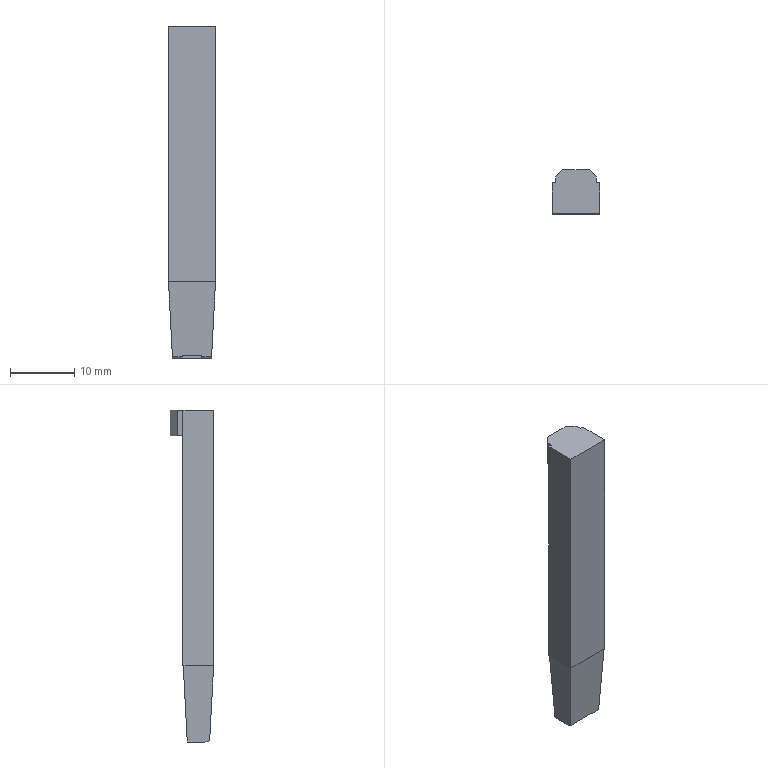Part | Creo | 1 solid | 23 faces | box 7.421 x 6.821 x 51.658 mm | volume 1794 mm3 | plane 23
STEP:
#1=CARTESIAN_POINT('',(0.,0.,0.));
#2=DIRECTION('',(0.,0.,1.));
#3=DIRECTION('',(1.,0.,0.));
#4=AXIS2_PLACEMENT_3D('',#1,#2,#3);
#5=CARTESIAN_POINT('',(22.844,-82.165,46.111));
#6=VERTEX_POINT('',#5);
#7=CARTESIAN_POINT('',(22.844,-86.985,46.111));
#8=VERTEX_POINT('',#7);
#9=CARTESIAN_POINT('',(22.844,-82.165,46.111));
#10=DIRECTION('',(0.,-1.,0.));
#11=VECTOR('',#10,4.821);
#12=LINE('',#9,#11);
#13=EDGE_CURVE('',#6,#8,#12,.T.);
#14=ORIENTED_EDGE('',*,*,#13,.T.);
#15=CARTESIAN_POINT('',(30.265,-86.985,46.111));
#16=VERTEX_POINT('',#15);
#17=CARTESIAN_POINT('',(30.265,-86.985,46.111));
#18=DIRECTION('',(-1.,0.,0.));
#19=VECTOR('',#18,7.421);
#20=LINE('',#17,#19);
#21=EDGE_CURVE('',#16,#8,#20,.T.);
#22=ORIENTED_EDGE('',*,*,#21,.F.);
#23=CARTESIAN_POINT('',(30.265,-82.165,46.111));
#24=VERTEX_POINT('',#23);
#25=CARTESIAN_POINT('',(30.265,-86.985,46.111));
#26=DIRECTION('',(0.,1.,0.));
#27=VECTOR('',#26,4.821);
#28=LINE('',#25,#27);
#29=EDGE_CURVE('',#16,#24,#28,.T.);
#30=ORIENTED_EDGE('',*,*,#29,.T.);
#31=CARTESIAN_POINT('',(30.265,-82.165,46.111));
#32=DIRECTION('',(-1.,0.,0.));
#33=VECTOR('',#32,7.421);
#34=LINE('',#31,#33);
#35=EDGE_CURVE('',#24,#6,#34,.T.);
#36=ORIENTED_EDGE('',*,*,#35,.T.);
#37=EDGE_LOOP('',(#14,#22,#30,#36));
#38=FACE_OUTER_BOUND('',#37,.F.);
#39=CARTESIAN_POINT('',(30.215,-82.215,46.111));
#40=VERTEX_POINT('',#39);
#41=CARTESIAN_POINT('',(22.894,-82.215,46.111));
#42=VERTEX_POINT('',#41);
#43=CARTESIAN_POINT('',(30.215,-82.215,46.111));
#44=DIRECTION('',(-1.,0.,0.));
#45=VECTOR('',#44,7.321);
#46=LINE('',#43,#45);
#47=EDGE_CURVE('',#40,#42,#46,.T.);
#48=ORIENTED_EDGE('',*,*,#47,.F.);
#49=CARTESIAN_POINT('',(30.215,-86.935,46.111));
#50=VERTEX_POINT('',#49);
#51=CARTESIAN_POINT('',(30.215,-86.935,46.111));
#52=DIRECTION('',(0.,1.,0.));
#53=VECTOR('',#52,4.721);
#54=LINE('',#51,#53);
#55=EDGE_CURVE('',#50,#40,#54,.T.);
#56=ORIENTED_EDGE('',*,*,#55,.F.);
#57=CARTESIAN_POINT('',(22.894,-86.935,46.111));
#58=VERTEX_POINT('',#57);
#59=CARTESIAN_POINT('',(22.894,-86.935,46.111));
#60=DIRECTION('',(1.,0.,0.));
#61=VECTOR('',#60,7.321);
#62=LINE('',#59,#61);
#63=EDGE_CURVE('',#58,#50,#62,.T.);
#64=ORIENTED_EDGE('',*,*,#63,.F.);
#65=CARTESIAN_POINT('',(22.894,-82.215,46.111));
#66=DIRECTION('',(0.,-1.,0.));
#67=VECTOR('',#66,4.721);
#68=LINE('',#65,#67);
#69=EDGE_CURVE('',#42,#58,#68,.T.);
#70=ORIENTED_EDGE('',*,*,#69,.F.);
#71=EDGE_LOOP('',(#48,#56,#64,#70));
#72=FACE_BOUND('',#71,.F.);
#73=CARTESIAN_POINT('',(26.554,-82.215,46.111));
#74=DIRECTION('',(0.,0.,1.));
#75=DIRECTION('',(1.,0.,0.));
#76=AXIS2_PLACEMENT_3D('',#73,#74,#75);
#77=PLANE('',#76);
#78=ADVANCED_FACE('',(#38,#72),#77,.F.);
#79=ORIENTED_EDGE('',*,*,#13,.F.);
#80=CARTESIAN_POINT('',(22.844,-82.165,85.91));
#81=VERTEX_POINT('',#80);
#82=CARTESIAN_POINT('',(22.844,-82.165,85.91));
#83=DIRECTION('',(0.,0.,-1.));
#84=VECTOR('',#83,39.799);
#85=LINE('',#82,#84);
#86=EDGE_CURVE('',#81,#6,#85,.T.);
#87=ORIENTED_EDGE('',*,*,#86,.F.);
#88=CARTESIAN_POINT('',(22.844,-86.985,85.91));
#89=VERTEX_POINT('',#88);
#90=CARTESIAN_POINT('',(22.844,-82.165,85.91));
#91=DIRECTION('',(0.,-1.,0.));
#92=VECTOR('',#91,4.821);
#93=LINE('',#90,#92);
#94=EDGE_CURVE('',#81,#89,#93,.T.);
#95=ORIENTED_EDGE('',*,*,#94,.T.);
#96=CARTESIAN_POINT('',(22.844,-86.985,85.91));
#97=DIRECTION('',(0.,0.,-1.));
#98=VECTOR('',#97,39.799);
#99=LINE('',#96,#98);
#100=EDGE_CURVE('',#89,#8,#99,.T.);
#101=ORIENTED_EDGE('',*,*,#100,.T.);
#102=EDGE_LOOP('',(#79,#87,#95,#101));
#103=FACE_OUTER_BOUND('',#102,.F.);
#104=CARTESIAN_POINT('',(22.844,-84.575,30.111));
#105=DIRECTION('',(-1.,0.,0.));
#106=DIRECTION('',(0.,0.,1.));
#107=AXIS2_PLACEMENT_3D('',#104,#105,#106);
#108=PLANE('',#107);
#109=ADVANCED_FACE('',(#103),#108,.T.);
#110=ORIENTED_EDGE('',*,*,#35,.F.);
#111=CARTESIAN_POINT('',(30.265,-82.165,85.91));
#112=VERTEX_POINT('',#111);
#113=CARTESIAN_POINT('',(30.265,-82.165,85.91));
#114=DIRECTION('',(0.,0.,-1.));
#115=VECTOR('',#114,39.799);
#116=LINE('',#113,#115);
#117=EDGE_CURVE('',#112,#24,#116,.T.);
#118=ORIENTED_EDGE('',*,*,#117,.F.);
#119=CARTESIAN_POINT('',(29.715,-82.165,85.91));
#120=VERTEX_POINT('',#119);
#121=CARTESIAN_POINT('',(30.265,-82.165,85.91));
#122=DIRECTION('',(-1.,0.,0.));
#123=VECTOR('',#122,0.55);
#124=LINE('',#121,#123);
#125=EDGE_CURVE('',#112,#120,#124,.T.);
#126=ORIENTED_EDGE('',*,*,#125,.T.);
#127=CARTESIAN_POINT('',(29.715,-82.165,81.91));
#128=VERTEX_POINT('',#127);
#129=CARTESIAN_POINT('',(29.715,-82.165,81.91));
#130=DIRECTION('',(0.,0.,1.));
#131=VECTOR('',#130,4.);
#132=LINE('',#129,#131);
#133=EDGE_CURVE('',#128,#120,#132,.T.);
#134=ORIENTED_EDGE('',*,*,#133,.F.);
#135=CARTESIAN_POINT('',(23.394,-82.165,81.91));
#136=VERTEX_POINT('',#135);
#137=CARTESIAN_POINT('',(23.394,-82.165,81.91));
#138=DIRECTION('',(1.,0.,0.));
#139=VECTOR('',#138,6.321);
#140=LINE('',#137,#139);
#141=EDGE_CURVE('',#136,#128,#140,.T.);
#142=ORIENTED_EDGE('',*,*,#141,.F.);
#143=CARTESIAN_POINT('',(23.394,-82.165,85.91));
#144=VERTEX_POINT('',#143);
#145=CARTESIAN_POINT('',(23.394,-82.165,85.91));
#146=DIRECTION('',(0.,0.,-1.));
#147=VECTOR('',#146,4.);
#148=LINE('',#145,#147);
#149=EDGE_CURVE('',#144,#136,#148,.T.);
#150=ORIENTED_EDGE('',*,*,#149,.F.);
#151=CARTESIAN_POINT('',(23.394,-82.165,85.91));
#152=DIRECTION('',(-1.,0.,0.));
#153=VECTOR('',#152,0.55);
#154=LINE('',#151,#153);
#155=EDGE_CURVE('',#144,#81,#154,.T.);
#156=ORIENTED_EDGE('',*,*,#155,.T.);
#157=ORIENTED_EDGE('',*,*,#86,.T.);
#158=EDGE_LOOP('',(#110,#118,#126,#134,#142,#150,#156,#157));
#159=FACE_OUTER_BOUND('',#158,.F.);
#160=CARTESIAN_POINT('',(26.554,-82.165,30.111));
#161=DIRECTION('',(0.,1.,0.));
#162=DIRECTION('',(0.,0.,1.));
#163=AXIS2_PLACEMENT_3D('',#160,#161,#162);
#164=PLANE('',#163);
#165=ADVANCED_FACE('',(#159),#164,.T.);
#166=ORIENTED_EDGE('',*,*,#29,.F.);
#167=CARTESIAN_POINT('',(30.265,-86.985,85.91));
#168=VERTEX_POINT('',#167);
#169=CARTESIAN_POINT('',(30.265,-86.985,85.91));
#170=DIRECTION('',(0.,0.,-1.));
#171=VECTOR('',#170,39.799);
#172=LINE('',#169,#171);
#173=EDGE_CURVE('',#168,#16,#172,.T.);
#174=ORIENTED_EDGE('',*,*,#173,.F.);
#175=CARTESIAN_POINT('',(30.265,-86.985,85.91));
#176=DIRECTION('',(0.,1.,0.));
#177=VECTOR('',#176,4.821);
#178=LINE('',#175,#177);
#179=EDGE_CURVE('',#168,#112,#178,.T.);
#180=ORIENTED_EDGE('',*,*,#179,.T.);
#181=ORIENTED_EDGE('',*,*,#117,.T.);
#182=EDGE_LOOP('',(#166,#174,#180,#181));
#183=FACE_OUTER_BOUND('',#182,.F.);
#184=CARTESIAN_POINT('',(30.265,-84.575,30.111));
#185=DIRECTION('',(1.,0.,0.));
#186=DIRECTION('',(0.,0.,-1.));
#187=AXIS2_PLACEMENT_3D('',#184,#185,#186);
#188=PLANE('',#187);
#189=ADVANCED_FACE('',(#183),#188,.T.);
#190=ORIENTED_EDGE('',*,*,#21,.T.);
#191=ORIENTED_EDGE('',*,*,#100,.F.);
#192=CARTESIAN_POINT('',(22.844,-86.985,85.91));
#193=DIRECTION('',(1.,0.,0.));
#194=VECTOR('',#193,7.421);
#195=LINE('',#192,#194);
#196=EDGE_CURVE('',#89,#168,#195,.T.);
#197=ORIENTED_EDGE('',*,*,#196,.T.);
#198=ORIENTED_EDGE('',*,*,#173,.T.);
#199=EDGE_LOOP('',(#190,#191,#197,#198));
#200=FACE_OUTER_BOUND('',#199,.F.);
#201=CARTESIAN_POINT('',(26.554,-86.985,30.111));
#202=DIRECTION('',(0.,-1.,0.));
#203=DIRECTION('',(0.,0.,-1.));
#204=AXIS2_PLACEMENT_3D('',#201,#202,#203);
#205=PLANE('',#204);
#206=ADVANCED_FACE('',(#200),#205,.T.);
#207=CARTESIAN_POINT('',(29.715,-81.265,85.91));
#208=VERTEX_POINT('',#207);
#209=CARTESIAN_POINT('',(29.715,-82.165,85.91));
#210=DIRECTION('',(0.,1.,0.));
#211=VECTOR('',#210,0.9);
#212=LINE('',#209,#211);
#213=EDGE_CURVE('',#120,#208,#212,.T.);
#214=ORIENTED_EDGE('',*,*,#213,.F.);
#215=ORIENTED_EDGE('',*,*,#125,.F.);
#216=ORIENTED_EDGE('',*,*,#179,.F.);
#217=ORIENTED_EDGE('',*,*,#196,.F.);
#218=ORIENTED_EDGE('',*,*,#94,.F.);
#219=ORIENTED_EDGE('',*,*,#155,.F.);
#220=CARTESIAN_POINT('',(23.394,-81.265,85.91));
#221=VERTEX_POINT('',#220);
#222=CARTESIAN_POINT('',(23.394,-81.265,85.91));
#223=DIRECTION('',(0.,-1.,0.));
#224=VECTOR('',#223,0.9);
#225=LINE('',#222,#224);
#226=EDGE_CURVE('',#221,#144,#225,.T.);
#227=ORIENTED_EDGE('',*,*,#226,.F.);
#228=CARTESIAN_POINT('',(24.494,-80.165,85.91));
#229=VERTEX_POINT('',#228);
#230=CARTESIAN_POINT('',(24.494,-80.165,85.91));
#231=DIRECTION('',(-0.7071,-0.7071,0.));
#232=VECTOR('',#231,1.556);
#233=LINE('',#230,#232);
#234=EDGE_CURVE('',#229,#221,#233,.T.);
#235=ORIENTED_EDGE('',*,*,#234,.F.);
#236=CARTESIAN_POINT('',(28.615,-80.165,85.91));
#237=VERTEX_POINT('',#236);
#238=CARTESIAN_POINT('',(28.615,-80.165,85.91));
#239=DIRECTION('',(-1.,0.,0.));
#240=VECTOR('',#239,4.121);
#241=LINE('',#238,#240);
#242=EDGE_CURVE('',#237,#229,#241,.T.);
#243=ORIENTED_EDGE('',*,*,#242,.F.);
#244=CARTESIAN_POINT('',(29.715,-81.265,85.91));
#245=DIRECTION('',(-0.7071,0.7071,0.));
#246=VECTOR('',#245,1.556);
#247=LINE('',#244,#246);
#248=EDGE_CURVE('',#208,#237,#247,.T.);
#249=ORIENTED_EDGE('',*,*,#248,.F.);
#250=EDGE_LOOP('',(#214,#215,#216,#217,#218,#219,#227,#235,#243,#249));
#251=FACE_OUTER_BOUND('',#250,.F.);
#252=CARTESIAN_POINT('',(62.144,-0.4125,85.91));
#253=DIRECTION('',(0.,0.,1.));
#254=DIRECTION('',(0.,1.,0.));
#255=AXIS2_PLACEMENT_3D('',#252,#253,#254);
#256=PLANE('',#255);
#257=ADVANCED_FACE('',(#251),#256,.T.);
#258=CARTESIAN_POINT('',(29.715,-81.265,81.91));
#259=VERTEX_POINT('',#258);
#260=CARTESIAN_POINT('',(29.715,-81.265,81.91));
#261=DIRECTION('',(0.,-1.,0.));
#262=VECTOR('',#261,0.9);
#263=LINE('',#260,#262);
#264=EDGE_CURVE('',#259,#128,#263,.T.);
#265=ORIENTED_EDGE('',*,*,#264,.T.);
#266=ORIENTED_EDGE('',*,*,#133,.T.);
#267=ORIENTED_EDGE('',*,*,#213,.T.);
#268=CARTESIAN_POINT('',(29.715,-81.265,85.91));
#269=DIRECTION('',(0.,0.,-1.));
#270=VECTOR('',#269,4.);
#271=LINE('',#268,#270);
#272=EDGE_CURVE('',#208,#259,#271,.T.);
#273=ORIENTED_EDGE('',*,*,#272,.T.);
#274=EDGE_LOOP('',(#265,#266,#267,#273));
#275=FACE_OUTER_BOUND('',#274,.F.);
#276=CARTESIAN_POINT('',(29.715,-81.715,81.91));
#277=DIRECTION('',(1.,0.,0.));
#278=DIRECTION('',(0.,0.,-1.));
#279=AXIS2_PLACEMENT_3D('',#276,#277,#278);
#280=PLANE('',#279);
#281=ADVANCED_FACE('',(#275),#280,.T.);
#282=CARTESIAN_POINT('',(24.494,-80.165,81.91));
#283=VERTEX_POINT('',#282);
#284=CARTESIAN_POINT('',(28.615,-80.165,81.91));
#285=VERTEX_POINT('',#284);
#286=CARTESIAN_POINT('',(24.494,-80.165,81.91));
#287=DIRECTION('',(1.,0.,0.));
#288=VECTOR('',#287,4.121);
#289=LINE('',#286,#288);
#290=EDGE_CURVE('',#283,#285,#289,.T.);
#291=ORIENTED_EDGE('',*,*,#290,.F.);
#292=CARTESIAN_POINT('',(23.394,-81.265,81.91));
#293=VERTEX_POINT('',#292);
#294=CARTESIAN_POINT('',(23.394,-81.265,81.91));
#295=DIRECTION('',(0.7071,0.7071,0.));
#296=VECTOR('',#295,1.556);
#297=LINE('',#294,#296);
#298=EDGE_CURVE('',#293,#283,#297,.T.);
#299=ORIENTED_EDGE('',*,*,#298,.F.);
#300=CARTESIAN_POINT('',(23.394,-82.165,81.91));
#301=DIRECTION('',(0.,1.,0.));
#302=VECTOR('',#301,0.9);
#303=LINE('',#300,#302);
#304=EDGE_CURVE('',#136,#293,#303,.T.);
#305=ORIENTED_EDGE('',*,*,#304,.F.);
#306=ORIENTED_EDGE('',*,*,#141,.T.);
#307=ORIENTED_EDGE('',*,*,#264,.F.);
#308=CARTESIAN_POINT('',(28.615,-80.165,81.91));
#309=DIRECTION('',(0.7071,-0.7071,0.));
#310=VECTOR('',#309,1.556);
#311=LINE('',#308,#310);
#312=EDGE_CURVE('',#285,#259,#311,.T.);
#313=ORIENTED_EDGE('',*,*,#312,.F.);
#314=EDGE_LOOP('',(#291,#299,#305,#306,#307,#313));
#315=FACE_OUTER_BOUND('',#314,.F.);
#316=CARTESIAN_POINT('',(26.554,-81.715,81.91));
#317=DIRECTION('',(0.,0.,-1.));
#318=DIRECTION('',(-1.,0.,0.));
#319=AXIS2_PLACEMENT_3D('',#316,#317,#318);
#320=PLANE('',#319);
#321=ADVANCED_FACE('',(#315),#320,.T.);
#322=ORIENTED_EDGE('',*,*,#242,.T.);
#323=CARTESIAN_POINT('',(24.494,-80.165,85.91));
#324=DIRECTION('',(0.,0.,-1.));
#325=VECTOR('',#324,4.);
#326=LINE('',#323,#325);
#327=EDGE_CURVE('',#229,#283,#326,.T.);
#328=ORIENTED_EDGE('',*,*,#327,.T.);
#329=ORIENTED_EDGE('',*,*,#290,.T.);
#330=CARTESIAN_POINT('',(28.615,-80.165,81.91));
#331=DIRECTION('',(0.,0.,1.));
#332=VECTOR('',#331,4.);
#333=LINE('',#330,#332);
#334=EDGE_CURVE('',#285,#237,#333,.T.);
#335=ORIENTED_EDGE('',*,*,#334,.T.);
#336=EDGE_LOOP('',(#322,#328,#329,#335));
#337=FACE_OUTER_BOUND('',#336,.F.);
#338=CARTESIAN_POINT('',(26.554,-80.165,81.91));
#339=DIRECTION('',(0.,1.,0.));
#340=DIRECTION('',(0.,0.,1.));
#341=AXIS2_PLACEMENT_3D('',#338,#339,#340);
#342=PLANE('',#341);
#343=ADVANCED_FACE('',(#337),#342,.T.);
#344=ORIENTED_EDGE('',*,*,#298,.T.);
#345=ORIENTED_EDGE('',*,*,#327,.F.);
#346=ORIENTED_EDGE('',*,*,#234,.T.);
#347=CARTESIAN_POINT('',(23.394,-81.265,81.91));
#348=DIRECTION('',(0.,0.,1.));
#349=VECTOR('',#348,4.);
#350=LINE('',#347,#349);
#351=EDGE_CURVE('',#293,#221,#350,.T.);
#352=ORIENTED_EDGE('',*,*,#351,.F.);
#353=EDGE_LOOP('',(#344,#345,#346,#352));
#354=FACE_OUTER_BOUND('',#353,.F.);
#355=CARTESIAN_POINT('',(24.394,-80.265,81.91));
#356=DIRECTION('',(0.7071,-0.7071,0.));
#357=DIRECTION('',(0.,0.,1.));
#358=AXIS2_PLACEMENT_3D('',#355,#356,#357);
#359=PLANE('',#358);
#360=ADVANCED_FACE('',(#354),#359,.F.);
#361=ORIENTED_EDGE('',*,*,#226,.T.);
#362=ORIENTED_EDGE('',*,*,#149,.T.);
#363=ORIENTED_EDGE('',*,*,#304,.T.);
#364=ORIENTED_EDGE('',*,*,#351,.T.);
#365=EDGE_LOOP('',(#361,#362,#363,#364));
#366=FACE_OUTER_BOUND('',#365,.F.);
#367=CARTESIAN_POINT('',(23.394,-81.715,81.91));
#368=DIRECTION('',(-1.,0.,0.));
#369=DIRECTION('',(0.,0.,1.));
#370=AXIS2_PLACEMENT_3D('',#367,#368,#369);
#371=PLANE('',#370);
#372=ADVANCED_FACE('',(#366),#371,.T.);
#373=ORIENTED_EDGE('',*,*,#312,.T.);
#374=ORIENTED_EDGE('',*,*,#272,.F.);
#375=ORIENTED_EDGE('',*,*,#248,.T.);
#376=ORIENTED_EDGE('',*,*,#334,.F.);
#377=EDGE_LOOP('',(#373,#374,#375,#376));
#378=FACE_OUTER_BOUND('',#377,.F.);
#379=CARTESIAN_POINT('',(29.715,-81.265,81.91));
#380=DIRECTION('',(-0.7071,-0.7071,0.));
#381=DIRECTION('',(0.,0.,1.));
#382=AXIS2_PLACEMENT_3D('',#379,#380,#381);
#383=PLANE('',#382);
#384=ADVANCED_FACE('',(#378),#383,.F.);
#385=ORIENTED_EDGE('',*,*,#47,.T.);
#386=CARTESIAN_POINT('',(23.515,-82.836,34.252));
#387=VERTEX_POINT('',#386);
#388=CARTESIAN_POINT('',(22.894,-82.215,46.111));
#389=DIRECTION('',(0.05226,-0.05226,-0.9973));
#390=VECTOR('',#389,11.892);
#391=LINE('',#388,#390);
#392=EDGE_CURVE('',#42,#387,#391,.T.);
#393=ORIENTED_EDGE('',*,*,#392,.T.);
#394=CARTESIAN_POINT('',(29.593,-82.836,34.252));
#395=VERTEX_POINT('',#394);
#396=CARTESIAN_POINT('',(23.515,-82.836,34.252));
#397=DIRECTION('',(1.,0.,0.));
#398=VECTOR('',#397,6.078);
#399=LINE('',#396,#398);
#400=EDGE_CURVE('',#387,#395,#399,.T.);
#401=ORIENTED_EDGE('',*,*,#400,.T.);
#402=CARTESIAN_POINT('',(30.215,-82.215,46.111));
#403=DIRECTION('',(-0.05226,-0.05226,-0.9973));
#404=VECTOR('',#403,11.892);
#405=LINE('',#402,#404);
#406=EDGE_CURVE('',#40,#395,#405,.T.);
#407=ORIENTED_EDGE('',*,*,#406,.F.);
#408=EDGE_LOOP('',(#385,#393,#401,#407));
#409=FACE_OUTER_BOUND('',#408,.F.);
#410=CARTESIAN_POINT('',(33.184,-82.32,44.101));
#411=DIRECTION('',(0.,0.9986,-0.05234));
#412=DIRECTION('',(-1.,0.,0.));
#413=AXIS2_PLACEMENT_3D('',#410,#411,#412);
#414=PLANE('',#413);
#415=ADVANCED_FACE('',(#409),#414,.T.);
#416=ORIENTED_EDGE('',*,*,#69,.T.);
#417=CARTESIAN_POINT('',(23.505,-86.324,34.456));
#418=VERTEX_POINT('',#417);
#419=CARTESIAN_POINT('',(22.894,-86.935,46.111));
#420=DIRECTION('',(0.05226,0.05226,-0.9973));
#421=VECTOR('',#420,11.687);
#422=LINE('',#419,#421);
#423=EDGE_CURVE('',#58,#418,#422,.T.);
#424=ORIENTED_EDGE('',*,*,#423,.T.);
#425=CARTESIAN_POINT('',(23.515,-85.561,34.252));
#426=VERTEX_POINT('',#425);
#427=CARTESIAN_POINT('',(23.515,-85.561,34.252));
#428=DIRECTION('',(-0.01356,-0.9658,0.2588));
#429=VECTOR('',#428,0.79);
#430=LINE('',#427,#429);
#431=EDGE_CURVE('',#426,#418,#430,.T.);
#432=ORIENTED_EDGE('',*,*,#431,.F.);
#433=CARTESIAN_POINT('',(23.515,-85.561,34.252));
#434=DIRECTION('',(0.,1.,0.));
#435=VECTOR('',#434,2.725);
#436=LINE('',#433,#435);
#437=EDGE_CURVE('',#426,#387,#436,.T.);
#438=ORIENTED_EDGE('',*,*,#437,.T.);
#439=ORIENTED_EDGE('',*,*,#392,.F.);
#440=EDGE_LOOP('',(#416,#424,#432,#438,#439));
#441=FACE_OUTER_BOUND('',#440,.F.);
#442=CARTESIAN_POINT('',(23.489,-82.215,34.752));
#443=DIRECTION('',(-0.9986,0.,-0.05234));
#444=DIRECTION('',(0.,-1.,0.));
#445=AXIS2_PLACEMENT_3D('',#442,#443,#444);
#446=PLANE('',#445);
#447=ADVANCED_FACE('',(#441),#446,.T.);
#448=ORIENTED_EDGE('',*,*,#63,.T.);
#449=CARTESIAN_POINT('',(29.604,-86.325,34.464));
#450=VERTEX_POINT('',#449);
#451=CARTESIAN_POINT('',(30.215,-86.935,46.111));
#452=DIRECTION('',(-0.05226,0.05226,-0.9973));
#453=VECTOR('',#452,11.679);
#454=LINE('',#451,#453);
#455=EDGE_CURVE('',#50,#450,#454,.T.);
#456=ORIENTED_EDGE('',*,*,#455,.T.);
#457=CARTESIAN_POINT('',(28.051,-86.325,34.464));
#458=VERTEX_POINT('',#457);
#459=CARTESIAN_POINT('',(28.051,-86.325,34.464));
#460=DIRECTION('',(1.,0.,0.));
#461=VECTOR('',#460,1.554);
#462=LINE('',#459,#461);
#463=EDGE_CURVE('',#458,#450,#462,.T.);
#464=ORIENTED_EDGE('',*,*,#463,.F.);
#465=CARTESIAN_POINT('',(28.043,-86.332,34.605));
#466=VERTEX_POINT('',#465);
#467=CARTESIAN_POINT('',(28.051,-86.325,34.464));
#468=DIRECTION('',(-0.05226,-0.05226,0.9973));
#469=VECTOR('',#468,0.1411);
#470=LINE('',#467,#469);
#471=EDGE_CURVE('',#458,#466,#470,.T.);
#472=ORIENTED_EDGE('',*,*,#471,.T.);
#473=CARTESIAN_POINT('',(25.065,-86.332,34.605));
#474=VERTEX_POINT('',#473);
#475=CARTESIAN_POINT('',(25.065,-86.332,34.605));
#476=DIRECTION('',(1.,0.,0.));
#477=VECTOR('',#476,2.978);
#478=LINE('',#475,#477);
#479=EDGE_CURVE('',#474,#466,#478,.T.);
#480=ORIENTED_EDGE('',*,*,#479,.F.);
#481=CARTESIAN_POINT('',(25.057,-86.324,34.456));
#482=VERTEX_POINT('',#481);
#483=CARTESIAN_POINT('',(25.057,-86.324,34.456));
#484=DIRECTION('',(0.05226,-0.05226,0.9973));
#485=VECTOR('',#484,0.1485);
#486=LINE('',#483,#485);
#487=EDGE_CURVE('',#482,#474,#486,.T.);
#488=ORIENTED_EDGE('',*,*,#487,.F.);
#489=CARTESIAN_POINT('',(23.505,-86.324,34.456));
#490=DIRECTION('',(1.,0.,0.));
#491=VECTOR('',#490,1.553);
#492=LINE('',#489,#491);
#493=EDGE_CURVE('',#418,#482,#492,.T.);
#494=ORIENTED_EDGE('',*,*,#493,.F.);
#495=ORIENTED_EDGE('',*,*,#423,.F.);
#496=EDGE_LOOP('',(#448,#456,#464,#472,#480,#488,#494,#495));
#497=FACE_OUTER_BOUND('',#496,.F.);
#498=CARTESIAN_POINT('',(-32.335,-86.34,34.755));
#499=DIRECTION('',(0.,0.9986,0.05234));
#500=DIRECTION('',(1.,0.,0.));
#501=AXIS2_PLACEMENT_3D('',#498,#499,#500);
#502=PLANE('',#501);
#503=ADVANCED_FACE('',(#497),#502,.F.);
#504=ORIENTED_EDGE('',*,*,#55,.T.);
#505=ORIENTED_EDGE('',*,*,#406,.T.);
#506=CARTESIAN_POINT('',(29.593,-85.534,34.252));
#507=VERTEX_POINT('',#506);
#508=CARTESIAN_POINT('',(29.593,-82.836,34.252));
#509=DIRECTION('',(0.,-1.,0.));
#510=VECTOR('',#509,2.698);
#511=LINE('',#508,#510);
#512=EDGE_CURVE('',#395,#507,#511,.T.);
#513=ORIENTED_EDGE('',*,*,#512,.T.);
#514=CARTESIAN_POINT('',(29.604,-86.325,34.464));
#515=DIRECTION('',(-0.01356,0.9658,-0.2588));
#516=VECTOR('',#515,0.8185);
#517=LINE('',#514,#516);
#518=EDGE_CURVE('',#450,#507,#517,.T.);
#519=ORIENTED_EDGE('',*,*,#518,.F.);
#520=ORIENTED_EDGE('',*,*,#455,.F.);
#521=EDGE_LOOP('',(#504,#505,#513,#519,#520));
#522=FACE_OUTER_BOUND('',#521,.F.);
#523=CARTESIAN_POINT('',(29.619,-82.215,34.752));
#524=DIRECTION('',(0.9986,0.,-0.05234));
#525=DIRECTION('',(0.,-1.,0.));
#526=AXIS2_PLACEMENT_3D('',#523,#524,#525);
#527=PLANE('',#526);
#528=ADVANCED_FACE('',(#522),#527,.T.);
#529=CARTESIAN_POINT('',(25.047,-85.561,34.252));
#530=VERTEX_POINT('',#529);
#531=CARTESIAN_POINT('',(25.047,-83.828,34.252));
#532=VERTEX_POINT('',#531);
#533=CARTESIAN_POINT('',(25.047,-85.561,34.252));
#534=DIRECTION('',(0.,1.,0.));
#535=VECTOR('',#534,1.734);
#536=LINE('',#533,#535);
#537=EDGE_CURVE('',#530,#532,#536,.T.);
#538=ORIENTED_EDGE('',*,*,#537,.T.);
#539=CARTESIAN_POINT('',(28.062,-83.828,34.252));
#540=VERTEX_POINT('',#539);
#541=CARTESIAN_POINT('',(28.062,-83.828,34.252));
#542=DIRECTION('',(-1.,0.,0.));
#543=VECTOR('',#542,3.015);
#544=LINE('',#541,#543);
#545=EDGE_CURVE('',#540,#532,#544,.T.);
#546=ORIENTED_EDGE('',*,*,#545,.F.);
#547=CARTESIAN_POINT('',(28.062,-85.535,34.252));
#548=VERTEX_POINT('',#547);
#549=CARTESIAN_POINT('',(28.062,-83.828,34.252));
#550=DIRECTION('',(-0.000001509,-1.,0.0000288));
#551=VECTOR('',#550,1.707);
#552=LINE('',#549,#551);
#553=EDGE_CURVE('',#540,#548,#552,.T.);
#554=ORIENTED_EDGE('',*,*,#553,.T.);
#555=CARTESIAN_POINT('',(29.593,-85.534,34.252));
#556=DIRECTION('',(-1.,-0.0002396,0.0000321));
#557=VECTOR('',#556,1.531);
#558=LINE('',#555,#557);
#559=EDGE_CURVE('',#507,#548,#558,.T.);
#560=ORIENTED_EDGE('',*,*,#559,.F.);
#561=ORIENTED_EDGE('',*,*,#512,.F.);
#562=ORIENTED_EDGE('',*,*,#400,.F.);
#563=ORIENTED_EDGE('',*,*,#437,.F.);
#564=CARTESIAN_POINT('',(25.047,-85.561,34.252));
#565=DIRECTION('',(-1.,0.,0.));
#566=VECTOR('',#565,1.531);
#567=LINE('',#564,#566);
#568=EDGE_CURVE('',#530,#426,#567,.T.);
#569=ORIENTED_EDGE('',*,*,#568,.F.);
#570=EDGE_LOOP('',(#538,#546,#554,#560,#561,#562,#563,#569));
#571=FACE_OUTER_BOUND('',#570,.F.);
#572=CARTESIAN_POINT('',(-28.218,-83.828,34.252));
#573=DIRECTION('',(0.,0.,1.));
#574=DIRECTION('',(0.,1.,0.));
#575=AXIS2_PLACEMENT_3D('',#572,#573,#574);
#576=PLANE('',#575);
#577=ADVANCED_FACE('',(#571),#576,.F.);
#578=CARTESIAN_POINT('',(25.065,-83.846,34.605));
#579=VERTEX_POINT('',#578);
#580=CARTESIAN_POINT('',(25.065,-83.846,34.605));
#581=DIRECTION('',(0.,-1.,0.));
#582=VECTOR('',#581,2.486);
#583=LINE('',#580,#582);
#584=EDGE_CURVE('',#579,#474,#583,.T.);
#585=ORIENTED_EDGE('',*,*,#584,.F.);
#586=CARTESIAN_POINT('',(25.065,-83.846,34.605));
#587=DIRECTION('',(-0.05226,0.05226,-0.9973));
#588=VECTOR('',#587,0.3535);
#589=LINE('',#586,#588);
#590=EDGE_CURVE('',#579,#532,#589,.T.);
#591=ORIENTED_EDGE('',*,*,#590,.T.);
#592=ORIENTED_EDGE('',*,*,#537,.F.);
#593=CARTESIAN_POINT('',(25.047,-85.561,34.252));
#594=DIRECTION('',(0.01356,-0.9658,0.2588));
#595=VECTOR('',#594,0.79);
#596=LINE('',#593,#595);
#597=EDGE_CURVE('',#530,#482,#596,.T.);
#598=ORIENTED_EDGE('',*,*,#597,.T.);
#599=ORIENTED_EDGE('',*,*,#487,.T.);
#600=EDGE_LOOP('',(#585,#591,#592,#598,#599));
#601=FACE_OUTER_BOUND('',#600,.F.);
#602=CARTESIAN_POINT('',(25.047,-83.828,34.252));
#603=DIRECTION('',(0.9986,0.,-0.05234));
#604=DIRECTION('',(-0.05234,0.,-0.9986));
#605=AXIS2_PLACEMENT_3D('',#602,#603,#604);
#606=PLANE('',#605);
#607=ADVANCED_FACE('',(#601),#606,.T.);
#608=CARTESIAN_POINT('',(28.043,-83.846,34.605));
#609=VERTEX_POINT('',#608);
#610=CARTESIAN_POINT('',(28.043,-86.332,34.605));
#611=DIRECTION('',(0.,1.,0.));
#612=VECTOR('',#611,2.486);
#613=LINE('',#610,#612);
#614=EDGE_CURVE('',#466,#609,#613,.T.);
#615=ORIENTED_EDGE('',*,*,#614,.T.);
#616=CARTESIAN_POINT('',(28.043,-83.846,34.605));
#617=DIRECTION('',(-1.,0.,0.));
#618=VECTOR('',#617,2.978);
#619=LINE('',#616,#618);
#620=EDGE_CURVE('',#609,#579,#619,.T.);
#621=ORIENTED_EDGE('',*,*,#620,.T.);
#622=ORIENTED_EDGE('',*,*,#584,.T.);
#623=ORIENTED_EDGE('',*,*,#479,.T.);
#624=EDGE_LOOP('',(#615,#621,#622,#623));
#625=FACE_OUTER_BOUND('',#624,.F.);
#626=CARTESIAN_POINT('',(25.047,-88.35,34.605));
#627=DIRECTION('',(0.,0.,-1.));
#628=DIRECTION('',(-1.,0.,0.));
#629=AXIS2_PLACEMENT_3D('',#626,#627,#628);
#630=PLANE('',#629);
#631=ADVANCED_FACE('',(#625),#630,.T.);
#632=CARTESIAN_POINT('',(28.051,-86.325,34.464));
#633=DIRECTION('',(0.01357,0.9658,-0.2589));
#634=VECTOR('',#633,0.8182);
#635=LINE('',#632,#634);
#636=EDGE_CURVE('',#458,#548,#635,.T.);
#637=ORIENTED_EDGE('',*,*,#636,.T.);
#638=ORIENTED_EDGE('',*,*,#553,.F.);
#639=CARTESIAN_POINT('',(28.043,-83.846,34.605));
#640=DIRECTION('',(0.05226,0.05226,-0.9973));
#641=VECTOR('',#640,0.3535);
#642=LINE('',#639,#641);
#643=EDGE_CURVE('',#609,#540,#642,.T.);
#644=ORIENTED_EDGE('',*,*,#643,.F.);
#645=ORIENTED_EDGE('',*,*,#614,.F.);
#646=ORIENTED_EDGE('',*,*,#471,.F.);
#647=EDGE_LOOP('',(#637,#638,#644,#645,#646));
#648=FACE_OUTER_BOUND('',#647,.F.);
#649=CARTESIAN_POINT('',(28.062,-83.828,34.252));
#650=DIRECTION('',(-0.9986,0.,-0.05234));
#651=DIRECTION('',(-0.05234,0.,0.9986));
#652=AXIS2_PLACEMENT_3D('',#649,#650,#651);
#653=PLANE('',#652);
#654=ADVANCED_FACE('',(#648),#653,.T.);
#655=ORIENTED_EDGE('',*,*,#636,.F.);
#656=ORIENTED_EDGE('',*,*,#463,.T.);
#657=ORIENTED_EDGE('',*,*,#518,.T.);
#658=ORIENTED_EDGE('',*,*,#559,.T.);
#659=EDGE_LOOP('',(#655,#656,#657,#658));
#660=FACE_OUTER_BOUND('',#659,.F.);
#661=CARTESIAN_POINT('',(41.122,-86.469,34.502));
#662=DIRECTION('',(0.,0.2588,0.9659));
#663=DIRECTION('',(0.,0.9659,-0.2588));
#664=AXIS2_PLACEMENT_3D('',#661,#662,#663);
#665=PLANE('',#664);
#666=ADVANCED_FACE('',(#660),#665,.F.);
#667=ORIENTED_EDGE('',*,*,#590,.F.);
#668=ORIENTED_EDGE('',*,*,#620,.F.);
#669=ORIENTED_EDGE('',*,*,#643,.T.);
#670=ORIENTED_EDGE('',*,*,#545,.T.);
#671=EDGE_LOOP('',(#667,#668,#669,#670));
#672=FACE_OUTER_BOUND('',#671,.F.);
#673=CARTESIAN_POINT('',(25.047,-83.828,34.252));
#674=DIRECTION('',(0.,-0.9986,-0.05234));
#675=DIRECTION('',(0.,-0.05234,0.9986));
#676=AXIS2_PLACEMENT_3D('',#673,#674,#675);
#677=PLANE('',#676);
#678=ADVANCED_FACE('',(#672),#677,.T.);
#679=ORIENTED_EDGE('',*,*,#493,.T.);
#680=ORIENTED_EDGE('',*,*,#597,.F.);
#681=ORIENTED_EDGE('',*,*,#568,.T.);
#682=ORIENTED_EDGE('',*,*,#431,.T.);
#683=EDGE_LOOP('',(#679,#680,#681,#682));
#684=FACE_OUTER_BOUND('',#683,.F.);
#685=CARTESIAN_POINT('',(41.122,-86.47,34.496));
#686=DIRECTION('',(0.,0.2588,0.9659));
#687=DIRECTION('',(0.,0.9659,-0.2588));
#688=AXIS2_PLACEMENT_3D('',#685,#686,#687);
#689=PLANE('',#688);
#690=ADVANCED_FACE('',(#684),#689,.F.);
#691=CLOSED_SHELL('',(#78,#109,#165,#189,#206,#257,#281,#321,#343,#360,#372,#384,#415,#447,#503,#528,#577,#607,#631,#654,#666,#678,#690));
#692=MANIFOLD_SOLID_BREP('',#691);
#693=(LENGTH_UNIT()NAMED_UNIT(*)SI_UNIT(.MILLI.,.METRE.));
#694=UNCERTAINTY_MEASURE_WITH_UNIT(LENGTH_MEASURE(0.005263),#693,'','');
#695=(NAMED_UNIT(*)PLANE_ANGLE_UNIT()SI_UNIT($,.RADIAN.));
#696=PLANE_ANGLE_MEASURE_WITH_UNIT(PLANE_ANGLE_MEASURE(0.01745),#695);
#697=(CONVERSION_BASED_UNIT('DEGREE',#696)NAMED_UNIT(*)PLANE_ANGLE_UNIT());
#698=(NAMED_UNIT(*)SI_UNIT($,.STERADIAN.)SOLID_ANGLE_UNIT());
#699=(GEOMETRIC_REPRESENTATION_CONTEXT(3)GLOBAL_UNCERTAINTY_ASSIGNED_CONTEXT((#694))GLOBAL_UNIT_ASSIGNED_CONTEXT((#693,#697,#698))REPRESENTATION_CONTEXT('',''));
#700=ADVANCED_BREP_SHAPE_REPRESENTATION('',(#4,#692),#699);